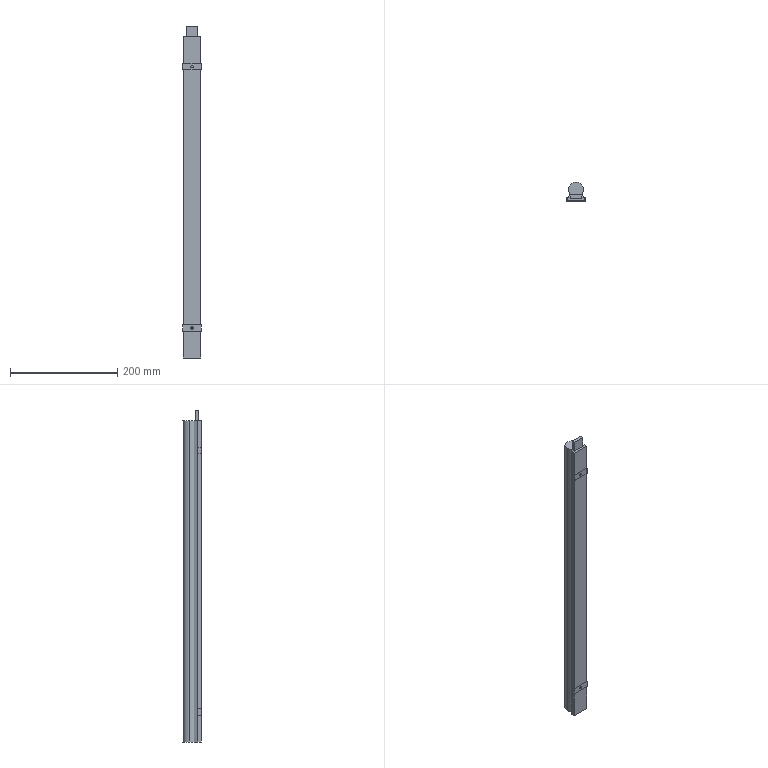Part | STEP file | T8 integrated LED tube_white 0.6m | 2 solids | 51 faces | box 34 x 35.5 x 620 mm | volume 542828 mm3 | plane 42 | cylinder 9 | commonest cylinder face diameters 4.5 x6 28 x3